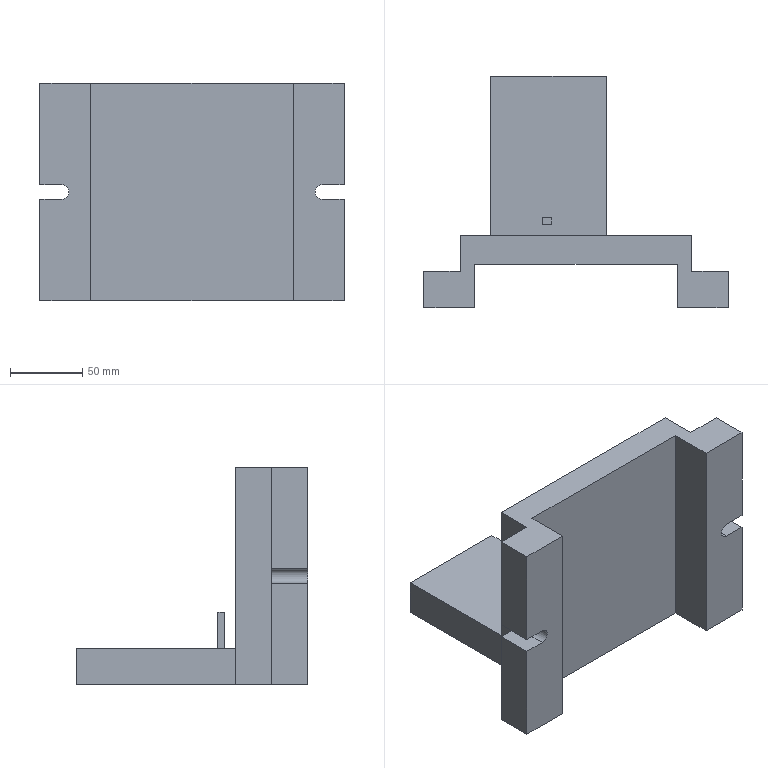Part | SolidWorks | features HoleWzd 3, ICE 3, Extrusion 1 | 1 solid | 87 faces | box 210 x 160 x 150 mm | volume 964186 mm3 | cylinder 30 | plane 29 | cone 28 | commonest cylinder face diameters 5 x24 6 x4 10 x2